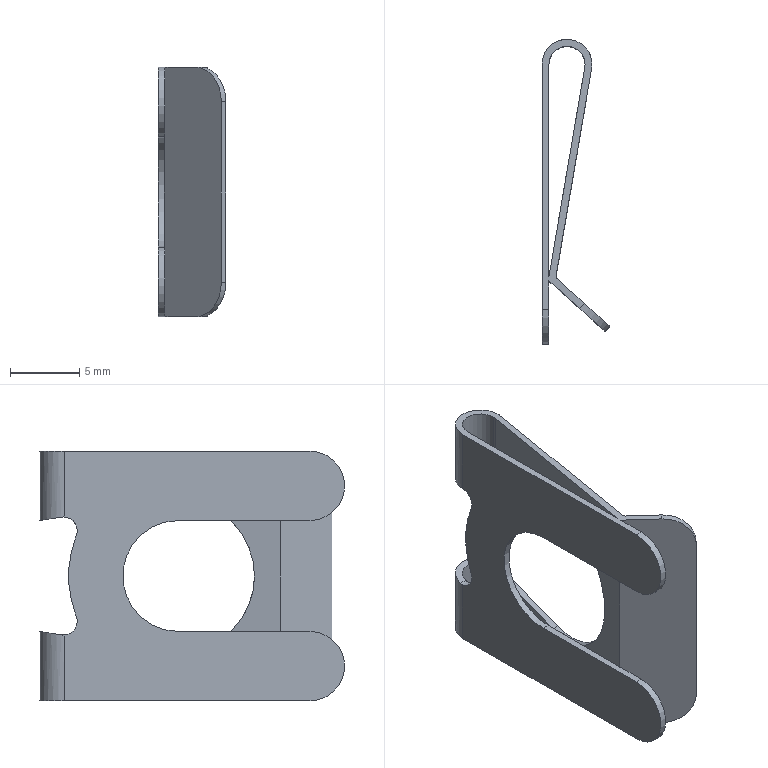Part | SolidWorks | features Fillet 2, BaseBody 1, ICE 1 | 1 solid | 36 faces | box 4.9 x 22 x 18 mm | volume 263.312 mm3 | cylinder 21 | plane 15 | commonest cylinder face diameters 2.6 x4 3.6 x4 5 x4 2 x3 11 x3 0.5 x1
STEP:
#1=CARTESIAN_POINT('',(0.5,8.2,-9.));
#2=VERTEX_POINT('',#1);
#3=CARTESIAN_POINT('',(3.1,8.2,-9.));
#4=VERTEX_POINT('',#3);
#5=CARTESIAN_POINT('',(1.8,8.2,-9.));
#6=DIRECTION('',(0.,0.,-1.));
#7=DIRECTION('',(1.,0.,0.));
#8=AXIS2_PLACEMENT_3D('',#5,#6,#7);
#9=CIRCLE('',#8,1.3);
#10=EDGE_CURVE('',#2,#4,#9,.T.);
#11=ORIENTED_EDGE('',*,*,#10,.T.);
#12=CARTESIAN_POINT('',(3.1,8.2,-4.282));
#13=VERTEX_POINT('',#12);
#14=CARTESIAN_POINT('',(3.1,8.2,9.));
#15=DIRECTION('',(0.,0.,1.));
#16=VECTOR('',#15,1000.);
#17=LINE('',#14,#16);
#18=EDGE_CURVE('',#4,#13,#17,.T.);
#19=ORIENTED_EDGE('',*,*,#18,.T.);
#20=CARTESIAN_POINT('',(0.5,8.2,-4.282));
#21=VERTEX_POINT('',#20);
#22=CARTESIAN_POINT('',(0.5,8.2,-4.282));
#23=CARTESIAN_POINT('',(0.5,10.8,-3.875));
#24=CARTESIAN_POINT('',(3.1,10.8,-3.875));
#25=CARTESIAN_POINT('',(3.1,8.2,-4.282));
#26=(BOUNDED_CURVE()B_SPLINE_CURVE(3,(#22,#23,#24,#25),.UNSPECIFIED.,.F.,.F.)B_SPLINE_CURVE_WITH_KNOTS((4,4),(4.712,7.854),.UNSPECIFIED.)CURVE()GEOMETRIC_REPRESENTATION_ITEM()RATIONAL_B_SPLINE_CURVE((1.,0.3333,0.3333,1.))REPRESENTATION_ITEM(''));
#27=EDGE_CURVE('',#21,#13,#26,.T.);
#28=ORIENTED_EDGE('',*,*,#27,.F.);
#29=CARTESIAN_POINT('',(0.5,8.2,9.));
#30=DIRECTION('',(0.,0.,-1.));
#31=VECTOR('',#30,1000.);
#32=LINE('',#29,#31);
#33=EDGE_CURVE('',#21,#2,#32,.T.);
#34=ORIENTED_EDGE('',*,*,#33,.T.);
#35=EDGE_LOOP('',(#11,#19,#28,#34));
#36=FACE_OUTER_BOUND('',#35,.T.);
#37=CARTESIAN_POINT('',(1.8,8.2,9.));
#38=DIRECTION('',(0.,0.,1.));
#39=DIRECTION('',(1.,0.,0.));
#40=AXIS2_PLACEMENT_3D('',#37,#38,#39);
#41=CYLINDRICAL_SURFACE('',#40,1.3);
#42=ADVANCED_FACE('',(#36),#41,.F.);
#43=CARTESIAN_POINT('',(0.5,8.437,4.245));
#44=VERTEX_POINT('',#43);
#45=CARTESIAN_POINT('',(0.5,8.283,4.257));
#46=VERTEX_POINT('',#45);
#47=CARTESIAN_POINT('',(0.5,8.283,3.257));
#48=DIRECTION('',(1.,0.,0.));
#49=DIRECTION('',(0.,0.,1.));
#50=AXIS2_PLACEMENT_3D('',#47,#48,#49);
#51=CIRCLE('',#50,1.);
#52=EDGE_CURVE('',#44,#46,#51,.T.);
#53=ORIENTED_EDGE('',*,*,#52,.T.);
#54=CARTESIAN_POINT('',(0.001899,8.283,4.257));
#55=VERTEX_POINT('',#54);
#56=CARTESIAN_POINT('',(-4.4,8.283,4.257));
#57=DIRECTION('',(-1.,0.,0.));
#58=VECTOR('',#57,1000.);
#59=LINE('',#56,#58);
#60=EDGE_CURVE('',#46,#55,#59,.T.);
#61=ORIENTED_EDGE('',*,*,#60,.T.);
#62=CARTESIAN_POINT('',(0.01573,8.437,4.245));
#63=VERTEX_POINT('',#62);
#64=CARTESIAN_POINT('',(0.01573,8.437,4.245));
#65=CARTESIAN_POINT('',(0.008933,8.386,4.253));
#66=CARTESIAN_POINT('',(0.004295,8.335,4.257));
#67=CARTESIAN_POINT('',(0.001899,8.283,4.257));
#68=B_SPLINE_CURVE_WITH_KNOTS('',3,(#64,#65,#66,#67),.UNSPECIFIED.,.F.,.F.,(4,4),(-0.0001563,0.),.UNSPECIFIED.);
#69=EDGE_CURVE('',#63,#55,#68,.T.);
#70=ORIENTED_EDGE('',*,*,#69,.F.);
#71=CARTESIAN_POINT('',(5.4,8.437,4.245));
#72=DIRECTION('',(-1.,0.,0.));
#73=VECTOR('',#72,1000.);
#74=LINE('',#71,#73);
#75=EDGE_CURVE('',#44,#63,#74,.T.);
#76=ORIENTED_EDGE('',*,*,#75,.F.);
#77=EDGE_LOOP('',(#53,#61,#70,#76));
#78=FACE_OUTER_BOUND('',#77,.T.);
#79=CARTESIAN_POINT('',(-4.4,8.283,3.257));
#80=DIRECTION('',(-1.,0.,0.));
#81=DIRECTION('',(0.,0.,1.));
#82=AXIS2_PLACEMENT_3D('',#79,#80,#81);
#83=CYLINDRICAL_SURFACE('',#82,1.);
#84=ADVANCED_FACE('',(#78),#83,.F.);
#85=CARTESIAN_POINT('',(3.1,8.2,4.282));
#86=VERTEX_POINT('',#85);
#87=CARTESIAN_POINT('',(0.5,8.2,4.282));
#88=VERTEX_POINT('',#87);
#89=CARTESIAN_POINT('',(3.1,8.2,4.282));
#90=CARTESIAN_POINT('',(3.1,10.8,3.875));
#91=CARTESIAN_POINT('',(0.5,10.8,3.875));
#92=CARTESIAN_POINT('',(0.5,8.2,4.282));
#93=(BOUNDED_CURVE()B_SPLINE_CURVE(3,(#89,#90,#91,#92),.UNSPECIFIED.,.F.,.F.)B_SPLINE_CURVE_WITH_KNOTS((4,4),(1.571,4.712),.UNSPECIFIED.)CURVE()GEOMETRIC_REPRESENTATION_ITEM()RATIONAL_B_SPLINE_CURVE((1.,0.3333,0.3333,1.))REPRESENTATION_ITEM(''));
#94=EDGE_CURVE('',#86,#88,#93,.T.);
#95=ORIENTED_EDGE('',*,*,#94,.F.);
#96=CARTESIAN_POINT('',(3.1,8.2,9.));
#97=VERTEX_POINT('',#96);
#98=CARTESIAN_POINT('',(3.1,8.2,9.));
#99=DIRECTION('',(0.,0.,1.));
#100=VECTOR('',#99,1000.);
#101=LINE('',#98,#100);
#102=EDGE_CURVE('',#86,#97,#101,.T.);
#103=ORIENTED_EDGE('',*,*,#102,.T.);
#104=CARTESIAN_POINT('',(0.5,8.2,9.));
#105=VERTEX_POINT('',#104);
#106=CARTESIAN_POINT('',(1.8,8.2,9.));
#107=DIRECTION('',(0.,0.,-1.));
#108=DIRECTION('',(1.,0.,0.));
#109=AXIS2_PLACEMENT_3D('',#106,#107,#108);
#110=CIRCLE('',#109,1.3);
#111=EDGE_CURVE('',#105,#97,#110,.T.);
#112=ORIENTED_EDGE('',*,*,#111,.F.);
#113=CARTESIAN_POINT('',(0.5,8.2,9.));
#114=DIRECTION('',(0.,0.,-1.));
#115=VECTOR('',#114,1000.);
#116=LINE('',#113,#115);
#117=EDGE_CURVE('',#105,#88,#116,.T.);
#118=ORIENTED_EDGE('',*,*,#117,.T.);
#119=EDGE_LOOP('',(#95,#103,#112,#118));
#120=FACE_OUTER_BOUND('',#119,.T.);
#121=CARTESIAN_POINT('',(1.8,8.2,9.));
#122=DIRECTION('',(0.,0.,1.));
#123=DIRECTION('',(1.,0.,0.));
#124=AXIS2_PLACEMENT_3D('',#121,#122,#123);
#125=CYLINDRICAL_SURFACE('',#124,1.3);
#126=ADVANCED_FACE('',(#120),#125,.F.);
#127=CARTESIAN_POINT('',(3.574,7.896,-9.));
#128=VERTEX_POINT('',#127);
#129=CARTESIAN_POINT('',(3.6,8.2,-9.));
#130=VERTEX_POINT('',#129);
#131=CARTESIAN_POINT('',(1.8,8.2,-9.));
#132=DIRECTION('',(0.,0.,1.));
#133=DIRECTION('',(1.,0.,0.));
#134=AXIS2_PLACEMENT_3D('',#131,#132,#133);
#135=CIRCLE('',#134,1.8);
#136=EDGE_CURVE('',#128,#130,#135,.T.);
#137=ORIENTED_EDGE('',*,*,#136,.T.);
#138=CARTESIAN_POINT('',(3.6,8.2,-4.282));
#139=VERTEX_POINT('',#138);
#140=CARTESIAN_POINT('',(3.6,8.2,9.));
#141=DIRECTION('',(0.,0.,1.));
#142=VECTOR('',#141,1000.);
#143=LINE('',#140,#142);
#144=EDGE_CURVE('',#130,#139,#143,.T.);
#145=ORIENTED_EDGE('',*,*,#144,.T.);
#146=CARTESIAN_POINT('',(3.574,7.896,-4.33));
#147=VERTEX_POINT('',#146);
#148=CARTESIAN_POINT('',(3.6,8.2,-4.282));
#149=CARTESIAN_POINT('',(3.6,8.098,-4.298));
#150=CARTESIAN_POINT('',(3.591,7.997,-4.314));
#151=CARTESIAN_POINT('',(3.574,7.896,-4.33));
#152=(BOUNDED_CURVE()B_SPLINE_CURVE(3,(#148,#149,#150,#151),.UNSPECIFIED.,.F.,.F.)B_SPLINE_CURVE_WITH_KNOTS((4,4),(1.571,1.74),.UNSPECIFIED.)CURVE()GEOMETRIC_REPRESENTATION_ITEM()RATIONAL_B_SPLINE_CURVE((1.,0.9976,0.9976,1.))REPRESENTATION_ITEM(''));
#153=EDGE_CURVE('',#139,#147,#152,.T.);
#154=ORIENTED_EDGE('',*,*,#153,.T.);
#155=CARTESIAN_POINT('',(3.574,7.896,9.));
#156=DIRECTION('',(0.,0.,-1.));
#157=VECTOR('',#156,1000.);
#158=LINE('',#155,#157);
#159=EDGE_CURVE('',#147,#128,#158,.T.);
#160=ORIENTED_EDGE('',*,*,#159,.T.);
#161=EDGE_LOOP('',(#137,#145,#154,#160));
#162=FACE_OUTER_BOUND('',#161,.T.);
#163=CARTESIAN_POINT('',(1.8,8.2,9.));
#164=DIRECTION('',(0.,0.,1.));
#165=DIRECTION('',(1.,0.,0.));
#166=AXIS2_PLACEMENT_3D('',#163,#164,#165);
#167=CYLINDRICAL_SURFACE('',#166,1.8);
#168=ADVANCED_FACE('',(#162),#167,.T.);
#169=CARTESIAN_POINT('',(3.6,8.2,4.282));
#170=VERTEX_POINT('',#169);
#171=CARTESIAN_POINT('',(3.574,7.896,4.33));
#172=VERTEX_POINT('',#171);
#173=CARTESIAN_POINT('',(3.6,8.2,4.282));
#174=CARTESIAN_POINT('',(3.6,8.098,4.298));
#175=CARTESIAN_POINT('',(3.591,7.997,4.314));
#176=CARTESIAN_POINT('',(3.574,7.896,4.33));
#177=(BOUNDED_CURVE()B_SPLINE_CURVE(3,(#173,#174,#175,#176),.UNSPECIFIED.,.F.,.F.)B_SPLINE_CURVE_WITH_KNOTS((4,4),(4.712,4.882),.UNSPECIFIED.)CURVE()GEOMETRIC_REPRESENTATION_ITEM()RATIONAL_B_SPLINE_CURVE((1.,0.9976,0.9976,1.))REPRESENTATION_ITEM(''));
#178=EDGE_CURVE('',#170,#172,#177,.T.);
#179=ORIENTED_EDGE('',*,*,#178,.F.);
#180=CARTESIAN_POINT('',(3.6,8.2,9.));
#181=VERTEX_POINT('',#180);
#182=CARTESIAN_POINT('',(3.6,8.2,9.));
#183=DIRECTION('',(0.,0.,1.));
#184=VECTOR('',#183,1000.);
#185=LINE('',#182,#184);
#186=EDGE_CURVE('',#170,#181,#185,.T.);
#187=ORIENTED_EDGE('',*,*,#186,.T.);
#188=CARTESIAN_POINT('',(3.574,7.896,9.));
#189=VERTEX_POINT('',#188);
#190=CARTESIAN_POINT('',(1.8,8.2,9.));
#191=DIRECTION('',(0.,0.,1.));
#192=DIRECTION('',(1.,0.,0.));
#193=AXIS2_PLACEMENT_3D('',#190,#191,#192);
#194=CIRCLE('',#193,1.8);
#195=EDGE_CURVE('',#189,#181,#194,.T.);
#196=ORIENTED_EDGE('',*,*,#195,.F.);
#197=CARTESIAN_POINT('',(3.574,7.896,9.));
#198=DIRECTION('',(0.,0.,-1.));
#199=VECTOR('',#198,1000.);
#200=LINE('',#197,#199);
#201=EDGE_CURVE('',#189,#172,#200,.T.);
#202=ORIENTED_EDGE('',*,*,#201,.T.);
#203=EDGE_LOOP('',(#179,#187,#196,#202));
#204=FACE_OUTER_BOUND('',#203,.T.);
#205=CARTESIAN_POINT('',(1.8,8.2,9.));
#206=DIRECTION('',(0.,0.,1.));
#207=DIRECTION('',(1.,0.,0.));
#208=AXIS2_PLACEMENT_3D('',#205,#206,#207);
#209=CYLINDRICAL_SURFACE('',#208,1.8);
#210=ADVANCED_FACE('',(#204),#209,.T.);
#211=CARTESIAN_POINT('',(1.715,0.,-5.5));
#212=VERTEX_POINT('',#211);
#213=CARTESIAN_POINT('',(1.715,0.,5.5));
#214=VERTEX_POINT('',#213);
#215=CARTESIAN_POINT('',(1.715,0.,-5.5));
#216=CARTESIAN_POINT('',(-0.1676,-11.,-5.5));
#217=CARTESIAN_POINT('',(-0.1676,-11.,5.5));
#218=CARTESIAN_POINT('',(1.715,0.,5.5));
#219=(BOUNDED_CURVE()B_SPLINE_CURVE(3,(#215,#216,#217,#218),.UNSPECIFIED.,.F.,.F.)B_SPLINE_CURVE_WITH_KNOTS((4,4),(1.571,4.712),.UNSPECIFIED.)CURVE()GEOMETRIC_REPRESENTATION_ITEM()RATIONAL_B_SPLINE_CURVE((1.,0.3333,0.3333,1.))REPRESENTATION_ITEM(''));
#220=EDGE_CURVE('',#212,#214,#219,.T.);
#221=ORIENTED_EDGE('',*,*,#220,.T.);
#222=CARTESIAN_POINT('',(2.223,0.,5.5));
#223=VERTEX_POINT('',#222);
#224=CARTESIAN_POINT('',(5.4,0.,5.5));
#225=DIRECTION('',(1.,0.,0.));
#226=VECTOR('',#225,1000.);
#227=LINE('',#224,#226);
#228=EDGE_CURVE('',#214,#223,#227,.T.);
#229=ORIENTED_EDGE('',*,*,#228,.T.);
#230=CARTESIAN_POINT('',(2.223,0.,-5.5));
#231=VERTEX_POINT('',#230);
#232=CARTESIAN_POINT('',(2.223,0.,5.5));
#233=CARTESIAN_POINT('',(0.3397,-11.,5.5));
#234=CARTESIAN_POINT('',(0.3397,-11.,-5.5));
#235=CARTESIAN_POINT('',(2.223,0.,-5.5));
#236=(BOUNDED_CURVE()B_SPLINE_CURVE(3,(#232,#233,#234,#235),.UNSPECIFIED.,.F.,.F.)B_SPLINE_CURVE_WITH_KNOTS((4,4),(1.571,4.712),.UNSPECIFIED.)CURVE()GEOMETRIC_REPRESENTATION_ITEM()RATIONAL_B_SPLINE_CURVE((1.,0.3333,0.3333,1.))REPRESENTATION_ITEM(''));
#237=EDGE_CURVE('',#223,#231,#236,.T.);
#238=ORIENTED_EDGE('',*,*,#237,.T.);
#239=CARTESIAN_POINT('',(5.4,0.,-5.5));
#240=DIRECTION('',(1.,0.,0.));
#241=VECTOR('',#240,1000.);
#242=LINE('',#239,#241);
#243=EDGE_CURVE('',#212,#231,#242,.T.);
#244=ORIENTED_EDGE('',*,*,#243,.F.);
#245=EDGE_LOOP('',(#221,#229,#238,#244));
#246=FACE_OUTER_BOUND('',#245,.T.);
#247=CARTESIAN_POINT('',(5.4,0.,0.));
#248=DIRECTION('',(1.,0.,0.));
#249=DIRECTION('',(0.,0.,-1.));
#250=AXIS2_PLACEMENT_3D('',#247,#248,#249);
#251=CYLINDRICAL_SURFACE('',#250,5.5);
#252=ADVANCED_FACE('',(#246),#251,.F.);
#253=CARTESIAN_POINT('',(1.861,0.8515,-5.434));
#254=VERTEX_POINT('',#253);
#255=CARTESIAN_POINT('',(1.861,0.8515,-5.434));
#256=CARTESIAN_POINT('',(1.813,0.5697,-5.478));
#257=CARTESIAN_POINT('',(1.764,0.2853,-5.5));
#258=CARTESIAN_POINT('',(1.715,0.,-5.5));
#259=(BOUNDED_CURVE()B_SPLINE_CURVE(3,(#255,#256,#257,#258),.UNSPECIFIED.,.F.,.F.)B_SPLINE_CURVE_WITH_KNOTS((4,4),(1.415,1.571),.UNSPECIFIED.)CURVE()GEOMETRIC_REPRESENTATION_ITEM()RATIONAL_B_SPLINE_CURVE((1.,0.998,0.998,1.))REPRESENTATION_ITEM(''));
#260=EDGE_CURVE('',#254,#212,#259,.T.);
#261=ORIENTED_EDGE('',*,*,#260,.T.);
#262=ORIENTED_EDGE('',*,*,#243,.T.);
#263=CARTESIAN_POINT('',(2.368,0.8515,-5.434));
#264=VERTEX_POINT('',#263);
#265=CARTESIAN_POINT('',(2.223,0.,-5.5));
#266=CARTESIAN_POINT('',(2.271,0.2853,-5.5));
#267=CARTESIAN_POINT('',(2.32,0.5697,-5.478));
#268=CARTESIAN_POINT('',(2.368,0.8515,-5.434));
#269=(BOUNDED_CURVE()B_SPLINE_CURVE(3,(#265,#266,#267,#268),.UNSPECIFIED.,.F.,.F.)B_SPLINE_CURVE_WITH_KNOTS((4,4),(4.712,4.868),.UNSPECIFIED.)CURVE()GEOMETRIC_REPRESENTATION_ITEM()RATIONAL_B_SPLINE_CURVE((1.,0.998,0.998,1.))REPRESENTATION_ITEM(''));
#270=EDGE_CURVE('',#231,#264,#269,.T.);
#271=ORIENTED_EDGE('',*,*,#270,.T.);
#272=CARTESIAN_POINT('',(5.4,0.8515,-5.434));
#273=DIRECTION('',(1.,0.,0.));
#274=VECTOR('',#273,1000.);
#275=LINE('',#272,#274);
#276=EDGE_CURVE('',#254,#264,#275,.T.);
#277=ORIENTED_EDGE('',*,*,#276,.F.);
#278=EDGE_LOOP('',(#261,#262,#271,#277));
#279=FACE_OUTER_BOUND('',#278,.T.);
#280=CARTESIAN_POINT('',(5.4,0.,0.));
#281=DIRECTION('',(1.,0.,0.));
#282=DIRECTION('',(0.,0.,-1.));
#283=AXIS2_PLACEMENT_3D('',#280,#281,#282);
#284=CYLINDRICAL_SURFACE('',#283,5.5);
#285=ADVANCED_FACE('',(#279),#284,.F.);
#286=CARTESIAN_POINT('',(4.565,-11.072,6.5));
#287=VERTEX_POINT('',#286);
#288=CARTESIAN_POINT('',(4.565,-11.072,-6.5));
#289=VERTEX_POINT('',#288);
#290=CARTESIAN_POINT('',(4.565,-11.072,-9.));
#291=DIRECTION('',(0.,0.,-1.));
#292=VECTOR('',#291,1000.);
#293=LINE('',#290,#292);
#294=EDGE_CURVE('',#287,#289,#293,.T.);
#295=ORIENTED_EDGE('',*,*,#294,.F.);
#296=CARTESIAN_POINT('',(2.707,-9.399,9.));
#297=VERTEX_POINT('',#296);
#298=CARTESIAN_POINT('',(2.707,-9.399,6.5));
#299=DIRECTION('',(-0.6689,-0.7434,0.));
#300=DIRECTION('',(-0.7434,0.6689,0.));
#301=AXIS2_PLACEMENT_3D('',#298,#299,#300);
#302=CIRCLE('',#301,2.5);
#303=EDGE_CURVE('',#287,#297,#302,.T.);
#304=ORIENTED_EDGE('',*,*,#303,.T.);
#305=CARTESIAN_POINT('',(0.5,-7.414,9.));
#306=VERTEX_POINT('',#305);
#307=CARTESIAN_POINT('',(0.7608,-7.648,9.));
#308=DIRECTION('',(0.7434,-0.6689,0.));
#309=VECTOR('',#308,1000.);
#310=LINE('',#307,#309);
#311=EDGE_CURVE('',#306,#297,#310,.T.);
#312=ORIENTED_EDGE('',*,*,#311,.F.);
#313=CARTESIAN_POINT('',(0.5,-7.414,4.));
#314=VERTEX_POINT('',#313);
#315=CARTESIAN_POINT('',(0.5,-7.414,9.));
#316=DIRECTION('',(0.,0.,1.));
#317=VECTOR('',#316,1000.);
#318=LINE('',#315,#317);
#319=EDGE_CURVE('',#314,#306,#318,.T.);
#320=ORIENTED_EDGE('',*,*,#319,.F.);
#321=CARTESIAN_POINT('',(0.4535,-7.372,4.));
#322=VERTEX_POINT('',#321);
#323=CARTESIAN_POINT('',(0.7608,-7.648,4.));
#324=DIRECTION('',(-0.7434,0.6689,0.));
#325=VECTOR('',#324,1000.);
#326=LINE('',#323,#325);
#327=EDGE_CURVE('',#314,#322,#326,.T.);
#328=ORIENTED_EDGE('',*,*,#327,.T.);
#329=CARTESIAN_POINT('',(0.4535,-7.372,-4.));
#330=VERTEX_POINT('',#329);
#331=CARTESIAN_POINT('',(0.4535,-7.372,9.));
#332=DIRECTION('',(0.,0.,-1.));
#333=VECTOR('',#332,1000.);
#334=LINE('',#331,#333);
#335=EDGE_CURVE('',#322,#330,#334,.T.);
#336=ORIENTED_EDGE('',*,*,#335,.T.);
#337=CARTESIAN_POINT('',(0.5,-7.414,-4.));
#338=VERTEX_POINT('',#337);
#339=CARTESIAN_POINT('',(0.7608,-7.648,-4.));
#340=DIRECTION('',(0.7434,-0.6689,0.));
#341=VECTOR('',#340,1000.);
#342=LINE('',#339,#341);
#343=EDGE_CURVE('',#330,#338,#342,.T.);
#344=ORIENTED_EDGE('',*,*,#343,.T.);
#345=CARTESIAN_POINT('',(0.5,-7.414,-9.));
#346=VERTEX_POINT('',#345);
#347=CARTESIAN_POINT('',(0.5,-7.414,9.));
#348=DIRECTION('',(0.,0.,1.));
#349=VECTOR('',#348,1000.);
#350=LINE('',#347,#349);
#351=EDGE_CURVE('',#346,#338,#350,.T.);
#352=ORIENTED_EDGE('',*,*,#351,.F.);
#353=CARTESIAN_POINT('',(2.707,-9.399,-9.));
#354=VERTEX_POINT('',#353);
#355=CARTESIAN_POINT('',(0.7608,-7.648,-9.));
#356=DIRECTION('',(0.7434,-0.6689,0.));
#357=VECTOR('',#356,1000.);
#358=LINE('',#355,#357);
#359=EDGE_CURVE('',#346,#354,#358,.T.);
#360=ORIENTED_EDGE('',*,*,#359,.T.);
#361=CARTESIAN_POINT('',(2.707,-9.399,-6.5));
#362=DIRECTION('',(-0.6689,-0.7434,0.));
#363=DIRECTION('',(-0.7434,0.6689,0.));
#364=AXIS2_PLACEMENT_3D('',#361,#362,#363);
#365=CIRCLE('',#364,2.5);
#366=EDGE_CURVE('',#354,#289,#365,.T.);
#367=ORIENTED_EDGE('',*,*,#366,.T.);
#368=EDGE_LOOP('',(#295,#304,#312,#320,#328,#336,#344,#352,#360,#367));
#369=FACE_OUTER_BOUND('',#368,.T.);
#370=CARTESIAN_POINT('',(0.7608,-7.648,9.));
#371=DIRECTION('',(0.6689,0.7434,0.));
#372=DIRECTION('',(0.,0.,-1.));
#373=AXIS2_PLACEMENT_3D('',#370,#371,#372);
#374=PLANE('',#373);
#375=ADVANCED_FACE('',(#369),#374,.F.);
#376=CARTESIAN_POINT('',(3.081,7.981,9.));
#377=VERTEX_POINT('',#376);
#378=CARTESIAN_POINT('',(0.5,-7.1,9.));
#379=VERTEX_POINT('',#378);
#380=CARTESIAN_POINT('',(3.081,7.981,9.));
#381=DIRECTION('',(-0.1687,-0.9857,0.));
#382=VECTOR('',#381,1000.);
#383=LINE('',#380,#382);
#384=EDGE_CURVE('',#377,#379,#383,.T.);
#385=ORIENTED_EDGE('',*,*,#384,.T.);
#386=CARTESIAN_POINT('',(0.5,-12.,9.));
#387=DIRECTION('',(0.,1.,0.));
#388=VECTOR('',#387,1000.);
#389=LINE('',#386,#388);
#390=EDGE_CURVE('',#379,#105,#389,.T.);
#391=ORIENTED_EDGE('',*,*,#390,.T.);
#392=ORIENTED_EDGE('',*,*,#111,.T.);
#393=CARTESIAN_POINT('',(1.8,8.2,9.));
#394=DIRECTION('',(0.,0.,-1.));
#395=DIRECTION('',(1.,0.,0.));
#396=AXIS2_PLACEMENT_3D('',#393,#394,#395);
#397=CIRCLE('',#396,1.3);
#398=EDGE_CURVE('',#97,#377,#397,.T.);
#399=ORIENTED_EDGE('',*,*,#398,.T.);
#400=EDGE_LOOP('',(#385,#391,#392,#399));
#401=FACE_BOUND('',#400,.T.);
#402=ORIENTED_EDGE('',*,*,#311,.T.);
#403=CARTESIAN_POINT('',(3.041,-9.028,9.));
#404=VERTEX_POINT('',#403);
#405=CARTESIAN_POINT('',(3.041,-9.028,9.));
#406=DIRECTION('',(0.6689,0.7434,0.));
#407=VECTOR('',#406,1000.);
#408=LINE('',#405,#407);
#409=EDGE_CURVE('',#297,#404,#408,.T.);
#410=ORIENTED_EDGE('',*,*,#409,.T.);
#411=CARTESIAN_POINT('',(1.095,-7.277,9.));
#412=VERTEX_POINT('',#411);
#413=CARTESIAN_POINT('',(4.9,-10.7,9.));
#414=DIRECTION('',(-0.7434,0.6689,0.));
#415=VECTOR('',#414,1000.);
#416=LINE('',#413,#415);
#417=EDGE_CURVE('',#404,#412,#416,.T.);
#418=ORIENTED_EDGE('',*,*,#417,.T.);
#419=CARTESIAN_POINT('',(1.016,-7.049,9.));
#420=VERTEX_POINT('',#419);
#421=CARTESIAN_POINT('',(1.263,-7.091,9.));
#422=DIRECTION('',(0.,0.,-1.));
#423=DIRECTION('',(1.,0.,0.));
#424=AXIS2_PLACEMENT_3D('',#421,#422,#423);
#425=CIRCLE('',#424,0.25);
#426=EDGE_CURVE('',#412,#420,#425,.T.);
#427=ORIENTED_EDGE('',*,*,#426,.T.);
#428=CARTESIAN_POINT('',(1.016,-7.049,9.));
#429=DIRECTION('',(0.1687,0.9857,0.));
#430=VECTOR('',#429,1000.);
#431=LINE('',#428,#430);
#432=EDGE_CURVE('',#420,#189,#431,.T.);
#433=ORIENTED_EDGE('',*,*,#432,.T.);
#434=ORIENTED_EDGE('',*,*,#195,.T.);
#435=CARTESIAN_POINT('',(0.,8.2,9.));
#436=VERTEX_POINT('',#435);
#437=CARTESIAN_POINT('',(1.8,8.2,9.));
#438=DIRECTION('',(0.,0.,1.));
#439=DIRECTION('',(1.,0.,0.));
#440=AXIS2_PLACEMENT_3D('',#437,#438,#439);
#441=CIRCLE('',#440,1.8);
#442=EDGE_CURVE('',#181,#436,#441,.T.);
#443=ORIENTED_EDGE('',*,*,#442,.T.);
#444=CARTESIAN_POINT('',(0.,-9.5,9.));
#445=VERTEX_POINT('',#444);
#446=CARTESIAN_POINT('',(0.,8.2,9.));
#447=DIRECTION('',(0.,-1.,0.));
#448=VECTOR('',#447,1000.);
#449=LINE('',#446,#448);
#450=EDGE_CURVE('',#436,#445,#449,.T.);
#451=ORIENTED_EDGE('',*,*,#450,.T.);
#452=CARTESIAN_POINT('',(0.5,-9.5,9.));
#453=VERTEX_POINT('',#452);
#454=CARTESIAN_POINT('',(1.8,-9.5,9.));
#455=DIRECTION('',(1.,0.,0.));
#456=VECTOR('',#455,1000.);
#457=LINE('',#454,#456);
#458=EDGE_CURVE('',#445,#453,#457,.T.);
#459=ORIENTED_EDGE('',*,*,#458,.T.);
#460=CARTESIAN_POINT('',(0.5,-12.,9.));
#461=DIRECTION('',(0.,1.,0.));
#462=VECTOR('',#461,1000.);
#463=LINE('',#460,#462);
#464=EDGE_CURVE('',#453,#306,#463,.T.);
#465=ORIENTED_EDGE('',*,*,#464,.T.);
#466=EDGE_LOOP('',(#402,#410,#418,#427,#433,#434,#443,#451,#459,#465));
#467=FACE_OUTER_BOUND('',#466,.T.);
#468=CARTESIAN_POINT('',(1.8,8.2,9.));
#469=DIRECTION('',(0.,0.,1.));
#470=DIRECTION('',(1.,0.,0.));
#471=AXIS2_PLACEMENT_3D('',#468,#469,#470);
#472=PLANE('',#471);
#473=ADVANCED_FACE('',(#401,#467),#472,.T.);
#474=CARTESIAN_POINT('',(0.5,-7.1,-9.));
#475=VERTEX_POINT('',#474);
#476=CARTESIAN_POINT('',(0.5,-12.,-9.));
#477=DIRECTION('',(0.,-1.,0.));
#478=VECTOR('',#477,1000.);
#479=LINE('',#476,#478);
#480=EDGE_CURVE('',#2,#475,#479,.T.);
#481=ORIENTED_EDGE('',*,*,#480,.T.);
#482=CARTESIAN_POINT('',(3.081,7.981,-9.));
#483=VERTEX_POINT('',#482);
#484=CARTESIAN_POINT('',(3.081,7.981,-9.));
#485=DIRECTION('',(-0.1687,-0.9857,0.));
#486=VECTOR('',#485,1000.);
#487=LINE('',#484,#486);
#488=EDGE_CURVE('',#483,#475,#487,.T.);
#489=ORIENTED_EDGE('',*,*,#488,.F.);
#490=CARTESIAN_POINT('',(1.8,8.2,-9.));
#491=DIRECTION('',(0.,0.,-1.));
#492=DIRECTION('',(1.,0.,0.));
#493=AXIS2_PLACEMENT_3D('',#490,#491,#492);
#494=CIRCLE('',#493,1.3);
#495=EDGE_CURVE('',#4,#483,#494,.T.);
#496=ORIENTED_EDGE('',*,*,#495,.F.);
#497=ORIENTED_EDGE('',*,*,#10,.F.);
#498=EDGE_LOOP('',(#481,#489,#496,#497));
#499=FACE_BOUND('',#498,.T.);
#500=CARTESIAN_POINT('',(3.041,-9.028,-9.));
#501=VERTEX_POINT('',#500);
#502=CARTESIAN_POINT('',(1.095,-7.277,-9.));
#503=VERTEX_POINT('',#502);
#504=CARTESIAN_POINT('',(4.9,-10.7,-9.));
#505=DIRECTION('',(-0.7434,0.6689,0.));
#506=VECTOR('',#505,1000.);
#507=LINE('',#504,#506);
#508=EDGE_CURVE('',#501,#503,#507,.T.);
#509=ORIENTED_EDGE('',*,*,#508,.F.);
#510=CARTESIAN_POINT('',(11.052,-0.1249,-9.));
#511=DIRECTION('',(-0.6689,-0.7434,0.));
#512=VECTOR('',#511,1000.);
#513=LINE('',#510,#512);
#514=EDGE_CURVE('',#501,#354,#513,.T.);
#515=ORIENTED_EDGE('',*,*,#514,.T.);
#516=ORIENTED_EDGE('',*,*,#359,.F.);
#517=CARTESIAN_POINT('',(0.5,-9.5,-9.));
#518=VERTEX_POINT('',#517);
#519=CARTESIAN_POINT('',(0.5,-12.,-9.));
#520=DIRECTION('',(0.,-1.,0.));
#521=VECTOR('',#520,1000.);
#522=LINE('',#519,#521);
#523=EDGE_CURVE('',#346,#518,#522,.T.);
#524=ORIENTED_EDGE('',*,*,#523,.T.);
#525=CARTESIAN_POINT('',(0.,-9.5,-9.));
#526=VERTEX_POINT('',#525);
#527=CARTESIAN_POINT('',(0.5,-9.5,-9.));
#528=DIRECTION('',(1.,0.,0.));
#529=VECTOR('',#528,1000.);
#530=LINE('',#527,#529);
#531=EDGE_CURVE('',#526,#518,#530,.T.);
#532=ORIENTED_EDGE('',*,*,#531,.F.);
#533=CARTESIAN_POINT('',(0.,8.2,-9.));
#534=VERTEX_POINT('',#533);
#535=CARTESIAN_POINT('',(0.,8.2,-9.));
#536=DIRECTION('',(0.,-1.,0.));
#537=VECTOR('',#536,1000.);
#538=LINE('',#535,#537);
#539=EDGE_CURVE('',#534,#526,#538,.T.);
#540=ORIENTED_EDGE('',*,*,#539,.F.);
#541=CARTESIAN_POINT('',(1.8,8.2,-9.));
#542=DIRECTION('',(0.,0.,1.));
#543=DIRECTION('',(1.,0.,0.));
#544=AXIS2_PLACEMENT_3D('',#541,#542,#543);
#545=CIRCLE('',#544,1.8);
#546=EDGE_CURVE('',#130,#534,#545,.T.);
#547=ORIENTED_EDGE('',*,*,#546,.F.);
#548=ORIENTED_EDGE('',*,*,#136,.F.);
#549=CARTESIAN_POINT('',(1.016,-7.049,-9.));
#550=VERTEX_POINT('',#549);
#551=CARTESIAN_POINT('',(1.016,-7.049,-9.));
#552=DIRECTION('',(0.1687,0.9857,0.));
#553=VECTOR('',#552,1000.);
#554=LINE('',#551,#553);
#555=EDGE_CURVE('',#550,#128,#554,.T.);
#556=ORIENTED_EDGE('',*,*,#555,.F.);
#557=CARTESIAN_POINT('',(1.263,-7.091,-9.));
#558=DIRECTION('',(0.,0.,1.));
#559=DIRECTION('',(1.,0.,0.));
#560=AXIS2_PLACEMENT_3D('',#557,#558,#559);
#561=CIRCLE('',#560,0.25);
#562=EDGE_CURVE('',#550,#503,#561,.T.);
#563=ORIENTED_EDGE('',*,*,#562,.T.);
#564=EDGE_LOOP('',(#509,#515,#516,#524,#532,#540,#547,#548,#556,#563));
#565=FACE_OUTER_BOUND('',#564,.T.);
#566=CARTESIAN_POINT('',(1.8,8.2,-9.));
#567=DIRECTION('',(0.,0.,1.));
#568=DIRECTION('',(1.,0.,0.));
#569=AXIS2_PLACEMENT_3D('',#566,#567,#568);
#570=PLANE('',#569);
#571=ADVANCED_FACE('',(#499,#565),#570,.F.);
#572=CARTESIAN_POINT('',(0.5,-7.1,-4.));
#573=VERTEX_POINT('',#572);
#574=CARTESIAN_POINT('',(-0.3149,-11.861,-4.));
#575=DIRECTION('',(0.1687,0.9857,0.));
#576=VECTOR('',#575,1000.);
#577=LINE('',#574,#576);
#578=EDGE_CURVE('',#330,#573,#577,.T.);
#579=ORIENTED_EDGE('',*,*,#578,.F.);
#580=ORIENTED_EDGE('',*,*,#335,.F.);
#581=CARTESIAN_POINT('',(0.5,-7.1,4.));
#582=VERTEX_POINT('',#581);
#583=CARTESIAN_POINT('',(1.681,-0.2021,4.));
#584=DIRECTION('',(-0.1687,-0.9857,0.));
#585=VECTOR('',#584,1000.);
#586=LINE('',#583,#585);
#587=EDGE_CURVE('',#582,#322,#586,.T.);
#588=ORIENTED_EDGE('',*,*,#587,.F.);
#589=CARTESIAN_POINT('',(0.5,-7.1,9.));
#590=DIRECTION('',(0.,0.,1.));
#591=VECTOR('',#590,1000.);
#592=LINE('',#589,#591);
#593=EDGE_CURVE('',#582,#379,#592,.T.);
#594=ORIENTED_EDGE('',*,*,#593,.T.);
#595=ORIENTED_EDGE('',*,*,#384,.F.);
#596=CARTESIAN_POINT('',(3.081,7.981,4.316));
#597=VERTEX_POINT('',#596);
#598=CARTESIAN_POINT('',(3.081,7.981,9.));
#599=DIRECTION('',(0.,0.,1.));
#600=VECTOR('',#599,1000.);
#601=LINE('',#598,#600);
#602=EDGE_CURVE('',#597,#377,#601,.T.);
#603=ORIENTED_EDGE('',*,*,#602,.F.);
#604=CARTESIAN_POINT('',(1.861,0.8515,5.434));
#605=VERTEX_POINT('',#604);
#606=CARTESIAN_POINT('',(1.861,0.8515,5.434));
#607=DIRECTION('',(0.1667,0.9741,-0.1527));
#608=VECTOR('',#607,1000.);
#609=LINE('',#606,#608);
#610=EDGE_CURVE('',#605,#597,#609,.T.);
#611=ORIENTED_EDGE('',*,*,#610,.F.);
#612=CARTESIAN_POINT('',(1.715,0.,5.5));
#613=CARTESIAN_POINT('',(1.764,0.2853,5.5));
#614=CARTESIAN_POINT('',(1.813,0.5697,5.478));
#615=CARTESIAN_POINT('',(1.861,0.8515,5.434));
#616=(BOUNDED_CURVE()B_SPLINE_CURVE(3,(#612,#613,#614,#615),.UNSPECIFIED.,.F.,.F.)B_SPLINE_CURVE_WITH_KNOTS((4,4),(4.712,4.868),.UNSPECIFIED.)CURVE()GEOMETRIC_REPRESENTATION_ITEM()RATIONAL_B_SPLINE_CURVE((1.,0.998,0.998,1.))REPRESENTATION_ITEM(''));
#617=EDGE_CURVE('',#214,#605,#616,.T.);
#618=ORIENTED_EDGE('',*,*,#617,.F.);
#619=ORIENTED_EDGE('',*,*,#220,.F.);
#620=ORIENTED_EDGE('',*,*,#260,.F.);
#621=CARTESIAN_POINT('',(3.081,7.981,-4.316));
#622=VERTEX_POINT('',#621);
#623=CARTESIAN_POINT('',(3.081,7.981,-4.316));
#624=DIRECTION('',(-0.1667,-0.9741,-0.1527));
#625=VECTOR('',#624,1000.);
#626=LINE('',#623,#625);
#627=EDGE_CURVE('',#622,#254,#626,.T.);
#628=ORIENTED_EDGE('',*,*,#627,.F.);
#629=CARTESIAN_POINT('',(3.081,7.981,9.));
#630=DIRECTION('',(0.,0.,1.));
#631=VECTOR('',#630,1000.);
#632=LINE('',#629,#631);
#633=EDGE_CURVE('',#483,#622,#632,.T.);
#634=ORIENTED_EDGE('',*,*,#633,.F.);
#635=ORIENTED_EDGE('',*,*,#488,.T.);
#636=CARTESIAN_POINT('',(0.5,-7.1,9.));
#637=DIRECTION('',(0.,0.,1.));
#638=VECTOR('',#637,1000.);
#639=LINE('',#636,#638);
#640=EDGE_CURVE('',#475,#573,#639,.T.);
#641=ORIENTED_EDGE('',*,*,#640,.T.);
#642=EDGE_LOOP('',(#579,#580,#588,#594,#595,#603,#611,#618,#619,#620,#628,#634,#635,#641));
#643=FACE_OUTER_BOUND('',#642,.T.);
#644=CARTESIAN_POINT('',(3.081,7.981,9.));
#645=DIRECTION('',(0.9857,-0.1687,0.));
#646=DIRECTION('',(0.,0.,-1.));
#647=AXIS2_PLACEMENT_3D('',#644,#645,#646);
#648=PLANE('',#647);
#649=ADVANCED_FACE('',(#643),#648,.F.);
#650=ORIENTED_EDGE('',*,*,#640,.F.);
#651=ORIENTED_EDGE('',*,*,#480,.F.);
#652=ORIENTED_EDGE('',*,*,#33,.F.);
#653=CARTESIAN_POINT('',(0.5,8.437,-4.245));
#654=VERTEX_POINT('',#653);
#655=CARTESIAN_POINT('',(0.5,0.8515,-5.434));
#656=DIRECTION('',(0.,-0.9879,-0.1548));
#657=VECTOR('',#656,1000.);
#658=LINE('',#655,#657);
#659=EDGE_CURVE('',#654,#21,#658,.T.);
#660=ORIENTED_EDGE('',*,*,#659,.F.);
#661=CARTESIAN_POINT('',(0.5,7.352,-2.891));
#662=VERTEX_POINT('',#661);
#663=CARTESIAN_POINT('',(0.5,8.283,-3.257));
#664=DIRECTION('',(1.,0.,0.));
#665=DIRECTION('',(0.,0.,1.));
#666=AXIS2_PLACEMENT_3D('',#663,#664,#665);
#667=CIRCLE('',#666,1.);
#668=EDGE_CURVE('',#662,#654,#667,.T.);
#669=ORIENTED_EDGE('',*,*,#668,.F.);
#670=CARTESIAN_POINT('',(0.5,7.352,2.891));
#671=VERTEX_POINT('',#670);
#672=CARTESIAN_POINT('',(0.5,0.,0.));
#673=DIRECTION('',(-1.,0.,0.));
#674=DIRECTION('',(0.,0.,1.));
#675=AXIS2_PLACEMENT_3D('',#672,#673,#674);
#676=CIRCLE('',#675,7.9);
#677=EDGE_CURVE('',#671,#662,#676,.T.);
#678=ORIENTED_EDGE('',*,*,#677,.F.);
#679=CARTESIAN_POINT('',(0.5,8.283,3.257));
#680=DIRECTION('',(1.,0.,0.));
#681=DIRECTION('',(0.,0.,1.));
#682=AXIS2_PLACEMENT_3D('',#679,#680,#681);
#683=CIRCLE('',#682,1.);
#684=EDGE_CURVE('',#46,#671,#683,.T.);
#685=ORIENTED_EDGE('',*,*,#684,.F.);
#686=ORIENTED_EDGE('',*,*,#52,.F.);
#687=CARTESIAN_POINT('',(0.5,10.,4.));
#688=DIRECTION('',(0.,0.9879,-0.1548));
#689=VECTOR('',#688,1000.);
#690=LINE('',#687,#689);
#691=EDGE_CURVE('',#88,#44,#690,.T.);
#692=ORIENTED_EDGE('',*,*,#691,.F.);
#693=ORIENTED_EDGE('',*,*,#117,.F.);
#694=ORIENTED_EDGE('',*,*,#390,.F.);
#695=ORIENTED_EDGE('',*,*,#593,.F.);
#696=CARTESIAN_POINT('',(0.5,0.,4.));
#697=VERTEX_POINT('',#696);
#698=CARTESIAN_POINT('',(0.5,-12.,4.));
#699=DIRECTION('',(0.,-1.,0.));
#700=VECTOR('',#699,1000.);
#701=LINE('',#698,#700);
#702=EDGE_CURVE('',#697,#582,#701,.T.);
#703=ORIENTED_EDGE('',*,*,#702,.F.);
#704=CARTESIAN_POINT('',(0.5,0.,-4.));
#705=VERTEX_POINT('',#704);
#706=CARTESIAN_POINT('',(0.5,0.,0.));
#707=DIRECTION('',(1.,0.,0.));
#708=DIRECTION('',(0.,0.,-1.));
#709=AXIS2_PLACEMENT_3D('',#706,#707,#708);
#710=CIRCLE('',#709,4.);
#711=EDGE_CURVE('',#705,#697,#710,.T.);
#712=ORIENTED_EDGE('',*,*,#711,.F.);
#713=CARTESIAN_POINT('',(0.5,-12.,-4.));
#714=DIRECTION('',(0.,1.,0.));
#715=VECTOR('',#714,1000.);
#716=LINE('',#713,#715);
#717=EDGE_CURVE('',#573,#705,#716,.T.);
#718=ORIENTED_EDGE('',*,*,#717,.F.);
#719=EDGE_LOOP('',(#650,#651,#652,#660,#669,#678,#685,#686,#692,#693,#694,#695,#703,#712,#718));
#720=FACE_OUTER_BOUND('',#719,.T.);
#721=CARTESIAN_POINT('',(0.5,-12.,9.));
#722=DIRECTION('',(-1.,0.,0.));
#723=DIRECTION('',(0.,0.,1.));
#724=AXIS2_PLACEMENT_3D('',#721,#722,#723);
#725=PLANE('',#724);
#726=ADVANCED_FACE('',(#720),#725,.F.);
#727=ORIENTED_EDGE('',*,*,#523,.F.);
#728=ORIENTED_EDGE('',*,*,#351,.T.);
#729=CARTESIAN_POINT('',(0.5,-9.5,-4.));
#730=VERTEX_POINT('',#729);
#731=CARTESIAN_POINT('',(0.5,-12.,-4.));
#732=DIRECTION('',(0.,1.,0.));
#733=VECTOR('',#732,1000.);
#734=LINE('',#731,#733);
#735=EDGE_CURVE('',#730,#338,#734,.T.);
#736=ORIENTED_EDGE('',*,*,#735,.F.);
#737=CARTESIAN_POINT('',(0.5,-9.5,-6.5));
#738=DIRECTION('',(-1.,0.,0.));
#739=DIRECTION('',(0.,0.,-1.));
#740=AXIS2_PLACEMENT_3D('',#737,#738,#739);
#741=CIRCLE('',#740,2.5);
#742=EDGE_CURVE('',#518,#730,#741,.T.);
#743=ORIENTED_EDGE('',*,*,#742,.F.);
#744=EDGE_LOOP('',(#727,#728,#736,#743));
#745=FACE_OUTER_BOUND('',#744,.T.);
#746=CARTESIAN_POINT('',(0.5,-12.,9.));
#747=DIRECTION('',(-1.,0.,0.));
#748=DIRECTION('',(0.,0.,1.));
#749=AXIS2_PLACEMENT_3D('',#746,#747,#748);
#750=PLANE('',#749);
#751=ADVANCED_FACE('',(#745),#750,.F.);
#752=CARTESIAN_POINT('',(2.368,0.8515,5.434));
#753=VERTEX_POINT('',#752);
#754=CARTESIAN_POINT('',(3.574,7.896,4.33));
#755=DIRECTION('',(-0.1667,-0.9741,0.1527));
#756=VECTOR('',#755,1000.);
#757=LINE('',#754,#756);
#758=EDGE_CURVE('',#172,#753,#757,.T.);
#759=ORIENTED_EDGE('',*,*,#758,.T.);
#760=CARTESIAN_POINT('',(5.4,0.8515,5.434));
#761=DIRECTION('',(-1.,0.,0.));
#762=VECTOR('',#761,1000.);
#763=LINE('',#760,#762);
#764=EDGE_CURVE('',#753,#605,#763,.T.);
#765=ORIENTED_EDGE('',*,*,#764,.T.);
#766=ORIENTED_EDGE('',*,*,#610,.T.);
#767=CARTESIAN_POINT('',(3.081,7.981,4.316));
#768=CARTESIAN_POINT('',(3.094,8.053,4.305));
#769=CARTESIAN_POINT('',(3.1,8.126,4.294));
#770=CARTESIAN_POINT('',(3.1,8.2,4.282));
#771=(BOUNDED_CURVE()B_SPLINE_CURVE(3,(#767,#768,#769,#770),.UNSPECIFIED.,.F.,.F.)B_SPLINE_CURVE_WITH_KNOTS((4,4),(1.401,1.571),.UNSPECIFIED.)CURVE()GEOMETRIC_REPRESENTATION_ITEM()RATIONAL_B_SPLINE_CURVE((1.,0.9976,0.9976,1.))REPRESENTATION_ITEM(''));
#772=EDGE_CURVE('',#597,#86,#771,.T.);
#773=ORIENTED_EDGE('',*,*,#772,.T.);
#774=ORIENTED_EDGE('',*,*,#94,.T.);
#775=ORIENTED_EDGE('',*,*,#691,.T.);
#776=ORIENTED_EDGE('',*,*,#75,.T.);
#777=CARTESIAN_POINT('',(0.01573,8.437,4.245));
#778=CARTESIAN_POINT('',(0.4343,11.582,3.752));
#779=CARTESIAN_POINT('',(3.6,11.373,3.785));
#780=CARTESIAN_POINT('',(3.6,8.2,4.282));
#781=(BOUNDED_CURVE()B_SPLINE_CURVE(3,(#777,#778,#779,#780),.UNSPECIFIED.,.F.,.F.)B_SPLINE_CURVE_WITH_KNOTS((4,4),(1.703,4.712),.UNSPECIFIED.)CURVE()GEOMETRIC_REPRESENTATION_ITEM()RATIONAL_B_SPLINE_CURVE((1.,0.3774,0.3774,1.))REPRESENTATION_ITEM(''));
#782=EDGE_CURVE('',#63,#170,#781,.T.);
#783=ORIENTED_EDGE('',*,*,#782,.T.);
#784=ORIENTED_EDGE('',*,*,#178,.T.);
#785=EDGE_LOOP('',(#759,#765,#766,#773,#774,#775,#776,#783,#784));
#786=FACE_OUTER_BOUND('',#785,.T.);
#787=CARTESIAN_POINT('',(5.4,10.,4.));
#788=DIRECTION('',(0.,-0.1548,-0.9879));
#789=DIRECTION('',(0.,-0.9879,0.1548));
#790=AXIS2_PLACEMENT_3D('',#787,#788,#789);
#791=PLANE('',#790);
#792=ADVANCED_FACE('',(#786),#791,.T.);
#793=CARTESIAN_POINT('',(0.01573,8.437,-4.245));
#794=VERTEX_POINT('',#793);
#795=CARTESIAN_POINT('',(0.01573,8.437,-4.245));
#796=CARTESIAN_POINT('',(0.4343,11.582,-3.752));
#797=CARTESIAN_POINT('',(3.6,11.373,-3.785));
#798=CARTESIAN_POINT('',(3.6,8.2,-4.282));
#799=(BOUNDED_CURVE()B_SPLINE_CURVE(3,(#795,#796,#797,#798),.UNSPECIFIED.,.F.,.F.)B_SPLINE_CURVE_WITH_KNOTS((4,4),(4.845,7.854),.UNSPECIFIED.)CURVE()GEOMETRIC_REPRESENTATION_ITEM()RATIONAL_B_SPLINE_CURVE((1.,0.3774,0.3774,1.))REPRESENTATION_ITEM(''));
#800=EDGE_CURVE('',#794,#139,#799,.T.);
#801=ORIENTED_EDGE('',*,*,#800,.F.);
#802=CARTESIAN_POINT('',(-4.4,8.437,-4.245));
#803=DIRECTION('',(1.,0.,0.));
#804=VECTOR('',#803,1000.);
#805=LINE('',#802,#804);
#806=EDGE_CURVE('',#794,#654,#805,.T.);
#807=ORIENTED_EDGE('',*,*,#806,.T.);
#808=ORIENTED_EDGE('',*,*,#659,.T.);
#809=ORIENTED_EDGE('',*,*,#27,.T.);
#810=CARTESIAN_POINT('',(3.1,8.2,-4.282));
#811=CARTESIAN_POINT('',(3.1,8.126,-4.294));
#812=CARTESIAN_POINT('',(3.094,8.053,-4.305));
#813=CARTESIAN_POINT('',(3.081,7.981,-4.316));
#814=(BOUNDED_CURVE()B_SPLINE_CURVE(3,(#810,#811,#812,#813),.UNSPECIFIED.,.F.,.F.)B_SPLINE_CURVE_WITH_KNOTS((4,4),(1.571,1.74),.UNSPECIFIED.)CURVE()GEOMETRIC_REPRESENTATION_ITEM()RATIONAL_B_SPLINE_CURVE((1.,0.9976,0.9976,1.))REPRESENTATION_ITEM(''));
#815=EDGE_CURVE('',#13,#622,#814,.T.);
#816=ORIENTED_EDGE('',*,*,#815,.T.);
#817=ORIENTED_EDGE('',*,*,#627,.T.);
#818=ORIENTED_EDGE('',*,*,#276,.T.);
#819=CARTESIAN_POINT('',(2.368,0.8515,-5.434));
#820=DIRECTION('',(0.1667,0.9741,0.1527));
#821=VECTOR('',#820,1000.);
#822=LINE('',#819,#821);
#823=EDGE_CURVE('',#264,#147,#822,.T.);
#824=ORIENTED_EDGE('',*,*,#823,.T.);
#825=ORIENTED_EDGE('',*,*,#153,.F.);
#826=EDGE_LOOP('',(#801,#807,#808,#809,#816,#817,#818,#824,#825));
#827=FACE_OUTER_BOUND('',#826,.T.);
#828=CARTESIAN_POINT('',(5.4,0.8515,-5.434));
#829=DIRECTION('',(0.,-0.1548,0.9879));
#830=DIRECTION('',(-1.,0.,0.));
#831=AXIS2_PLACEMENT_3D('',#828,#829,#830);
#832=PLANE('',#831);
#833=ADVANCED_FACE('',(#827),#832,.T.);
#834=ORIENTED_EDGE('',*,*,#432,.F.);
#835=CARTESIAN_POINT('',(1.016,-7.049,-9.));
#836=DIRECTION('',(0.,0.,-1.));
#837=VECTOR('',#836,1000.);
#838=LINE('',#835,#837);
#839=EDGE_CURVE('',#420,#550,#838,.T.);
#840=ORIENTED_EDGE('',*,*,#839,.T.);
#841=ORIENTED_EDGE('',*,*,#555,.T.);
#842=ORIENTED_EDGE('',*,*,#159,.F.);
#843=ORIENTED_EDGE('',*,*,#823,.F.);
#844=ORIENTED_EDGE('',*,*,#270,.F.);
#845=ORIENTED_EDGE('',*,*,#237,.F.);
#846=CARTESIAN_POINT('',(2.368,0.8515,5.434));
#847=CARTESIAN_POINT('',(2.32,0.5697,5.478));
#848=CARTESIAN_POINT('',(2.271,0.2853,5.5));
#849=CARTESIAN_POINT('',(2.223,0.,5.5));
#850=(BOUNDED_CURVE()B_SPLINE_CURVE(3,(#846,#847,#848,#849),.UNSPECIFIED.,.F.,.F.)B_SPLINE_CURVE_WITH_KNOTS((4,4),(1.415,1.571),.UNSPECIFIED.)CURVE()GEOMETRIC_REPRESENTATION_ITEM()RATIONAL_B_SPLINE_CURVE((1.,0.998,0.998,1.))REPRESENTATION_ITEM(''));
#851=EDGE_CURVE('',#753,#223,#850,.T.);
#852=ORIENTED_EDGE('',*,*,#851,.F.);
#853=ORIENTED_EDGE('',*,*,#758,.F.);
#854=ORIENTED_EDGE('',*,*,#201,.F.);
#855=EDGE_LOOP('',(#834,#840,#841,#842,#843,#844,#845,#852,#853,#854));
#856=FACE_OUTER_BOUND('',#855,.T.);
#857=CARTESIAN_POINT('',(1.016,-7.049,9.));
#858=DIRECTION('',(-0.9857,0.1687,0.));
#859=DIRECTION('',(0.,0.,1.));
#860=AXIS2_PLACEMENT_3D('',#857,#858,#859);
#861=PLANE('',#860);
#862=ADVANCED_FACE('',(#856),#861,.F.);
#863=ORIENTED_EDGE('',*,*,#450,.F.);
#864=CARTESIAN_POINT('',(0.,8.2,4.254));
#865=VERTEX_POINT('',#864);
#866=CARTESIAN_POINT('',(0.,8.2,9.));
#867=DIRECTION('',(0.,0.,1.));
#868=VECTOR('',#867,1000.);
#869=LINE('',#866,#868);
#870=EDGE_CURVE('',#865,#436,#869,.T.);
#871=ORIENTED_EDGE('',*,*,#870,.F.);
#872=CARTESIAN_POINT('',(0.,7.352,2.891));
#873=VERTEX_POINT('',#872);
#874=CARTESIAN_POINT('',(0.,8.283,3.257));
#875=DIRECTION('',(1.,0.,0.));
#876=DIRECTION('',(0.,0.,1.));
#877=AXIS2_PLACEMENT_3D('',#874,#875,#876);
#878=CIRCLE('',#877,1.);
#879=EDGE_CURVE('',#865,#873,#878,.T.);
#880=ORIENTED_EDGE('',*,*,#879,.T.);
#881=CARTESIAN_POINT('',(0.,7.352,-2.891));
#882=VERTEX_POINT('',#881);
#883=CARTESIAN_POINT('',(0.,0.,0.));
#884=DIRECTION('',(1.,0.,0.));
#885=DIRECTION('',(0.,0.,1.));
#886=AXIS2_PLACEMENT_3D('',#883,#884,#885);
#887=CIRCLE('',#886,7.9);
#888=EDGE_CURVE('',#882,#873,#887,.T.);
#889=ORIENTED_EDGE('',*,*,#888,.F.);
#890=CARTESIAN_POINT('',(0.,8.2,-4.254));
#891=VERTEX_POINT('',#890);
#892=CARTESIAN_POINT('',(0.,8.283,-3.257));
#893=DIRECTION('',(1.,0.,0.));
#894=DIRECTION('',(0.,0.,1.));
#895=AXIS2_PLACEMENT_3D('',#892,#893,#894);
#896=CIRCLE('',#895,1.);
#897=EDGE_CURVE('',#882,#891,#896,.T.);
#898=ORIENTED_EDGE('',*,*,#897,.T.);
#899=CARTESIAN_POINT('',(0.,8.2,9.));
#900=DIRECTION('',(0.,0.,1.));
#901=VECTOR('',#900,1000.);
#902=LINE('',#899,#901);
#903=EDGE_CURVE('',#534,#891,#902,.T.);
#904=ORIENTED_EDGE('',*,*,#903,.F.);
#905=ORIENTED_EDGE('',*,*,#539,.T.);
#906=CARTESIAN_POINT('',(0.,-9.5,-4.));
#907=VERTEX_POINT('',#906);
#908=CARTESIAN_POINT('',(0.,-9.5,-6.5));
#909=DIRECTION('',(1.,0.,0.));
#910=DIRECTION('',(0.,0.,-1.));
#911=AXIS2_PLACEMENT_3D('',#908,#909,#910);
#912=CIRCLE('',#911,2.5);
#913=EDGE_CURVE('',#907,#526,#912,.T.);
#914=ORIENTED_EDGE('',*,*,#913,.F.);
#915=CARTESIAN_POINT('',(0.,0.,-4.));
#916=VERTEX_POINT('',#915);
#917=CARTESIAN_POINT('',(0.,-12.,-4.));
#918=DIRECTION('',(0.,-1.,0.));
#919=VECTOR('',#918,1000.);
#920=LINE('',#917,#919);
#921=EDGE_CURVE('',#916,#907,#920,.T.);
#922=ORIENTED_EDGE('',*,*,#921,.F.);
#923=CARTESIAN_POINT('',(0.,0.,4.));
#924=VERTEX_POINT('',#923);
#925=CARTESIAN_POINT('',(0.,0.,0.));
#926=DIRECTION('',(1.,0.,0.));
#927=DIRECTION('',(0.,0.,-1.));
#928=AXIS2_PLACEMENT_3D('',#925,#926,#927);
#929=CIRCLE('',#928,4.);
#930=EDGE_CURVE('',#916,#924,#929,.T.);
#931=ORIENTED_EDGE('',*,*,#930,.T.);
#932=CARTESIAN_POINT('',(0.,-9.5,4.));
#933=VERTEX_POINT('',#932);
#934=CARTESIAN_POINT('',(0.,0.,4.));
#935=DIRECTION('',(0.,1.,0.));
#936=VECTOR('',#935,1000.);
#937=LINE('',#934,#936);
#938=EDGE_CURVE('',#933,#924,#937,.T.);
#939=ORIENTED_EDGE('',*,*,#938,.F.);
#940=CARTESIAN_POINT('',(0.,-9.5,6.5));
#941=DIRECTION('',(1.,0.,0.));
#942=DIRECTION('',(0.,0.,-1.));
#943=AXIS2_PLACEMENT_3D('',#940,#941,#942);
#944=CIRCLE('',#943,2.5);
#945=EDGE_CURVE('',#445,#933,#944,.T.);
#946=ORIENTED_EDGE('',*,*,#945,.F.);
#947=EDGE_LOOP('',(#863,#871,#880,#889,#898,#904,#905,#914,#922,#931,#939,#946));
#948=FACE_OUTER_BOUND('',#947,.T.);
#949=CARTESIAN_POINT('',(0.,8.2,9.));
#950=DIRECTION('',(1.,0.,0.));
#951=DIRECTION('',(0.,1.,0.));
#952=AXIS2_PLACEMENT_3D('',#949,#950,#951);
#953=PLANE('',#952);
#954=ADVANCED_FACE('',(#948),#953,.F.);
#955=ORIENTED_EDGE('',*,*,#945,.T.);
#956=CARTESIAN_POINT('',(0.5,-9.5,4.));
#957=VERTEX_POINT('',#956);
#958=CARTESIAN_POINT('',(0.5,-9.5,4.));
#959=DIRECTION('',(-1.,0.,0.));
#960=VECTOR('',#959,1000.);
#961=LINE('',#958,#960);
#962=EDGE_CURVE('',#957,#933,#961,.T.);
#963=ORIENTED_EDGE('',*,*,#962,.F.);
#964=CARTESIAN_POINT('',(0.5,-9.5,6.5));
#965=DIRECTION('',(-1.,0.,0.));
#966=DIRECTION('',(0.,0.,-1.));
#967=AXIS2_PLACEMENT_3D('',#964,#965,#966);
#968=CIRCLE('',#967,2.5);
#969=EDGE_CURVE('',#957,#453,#968,.T.);
#970=ORIENTED_EDGE('',*,*,#969,.T.);
#971=ORIENTED_EDGE('',*,*,#458,.F.);
#972=EDGE_LOOP('',(#955,#963,#970,#971));
#973=FACE_OUTER_BOUND('',#972,.T.);
#974=CARTESIAN_POINT('',(0.5,-9.5,6.5));
#975=DIRECTION('',(1.,0.,0.));
#976=DIRECTION('',(0.,0.,-1.));
#977=AXIS2_PLACEMENT_3D('',#974,#975,#976);
#978=CYLINDRICAL_SURFACE('',#977,2.5);
#979=ADVANCED_FACE('',(#973),#978,.T.);
#980=ORIENTED_EDGE('',*,*,#888,.T.);
#981=CARTESIAN_POINT('',(-4.4,7.352,2.891));
#982=DIRECTION('',(1.,0.,0.));
#983=VECTOR('',#982,1000.);
#984=LINE('',#981,#983);
#985=EDGE_CURVE('',#873,#671,#984,.T.);
#986=ORIENTED_EDGE('',*,*,#985,.T.);
#987=ORIENTED_EDGE('',*,*,#677,.T.);
#988=CARTESIAN_POINT('',(-4.4,7.352,-2.891));
#989=DIRECTION('',(-1.,0.,0.));
#990=VECTOR('',#989,1000.);
#991=LINE('',#988,#990);
#992=EDGE_CURVE('',#662,#882,#991,.T.);
#993=ORIENTED_EDGE('',*,*,#992,.T.);
#994=EDGE_LOOP('',(#980,#986,#987,#993));
#995=FACE_OUTER_BOUND('',#994,.T.);
#996=CARTESIAN_POINT('',(-4.4,0.,0.));
#997=DIRECTION('',(-1.,0.,0.));
#998=DIRECTION('',(0.,0.,1.));
#999=AXIS2_PLACEMENT_3D('',#996,#997,#998);
#1000=CYLINDRICAL_SURFACE('',#999,7.9);
#1001=ADVANCED_FACE('',(#995),#1000,.T.);
#1002=ORIENTED_EDGE('',*,*,#668,.T.);
#1003=ORIENTED_EDGE('',*,*,#806,.F.);
#1004=CARTESIAN_POINT('',(0.,8.2,-4.254));
#1005=CARTESIAN_POINT('',(0.,8.279,-4.26));
#1006=CARTESIAN_POINT('',(0.005255,8.359,-4.257));
#1007=CARTESIAN_POINT('',(0.01573,8.437,-4.245));
#1008=B_SPLINE_CURVE_WITH_KNOTS('',3,(#1004,#1005,#1006,#1007),.UNSPECIFIED.,.F.,.F.,(4,4),(0.,1.),.UNSPECIFIED.);
#1009=EDGE_CURVE('',#891,#794,#1008,.T.);
#1010=ORIENTED_EDGE('',*,*,#1009,.F.);
#1011=ORIENTED_EDGE('',*,*,#897,.F.);
#1012=ORIENTED_EDGE('',*,*,#992,.F.);
#1013=EDGE_LOOP('',(#1002,#1003,#1010,#1011,#1012));
#1014=FACE_OUTER_BOUND('',#1013,.T.);
#1015=CARTESIAN_POINT('',(-4.4,8.283,-3.257));
#1016=DIRECTION('',(-1.,0.,0.));
#1017=DIRECTION('',(0.,0.,1.));
#1018=AXIS2_PLACEMENT_3D('',#1015,#1016,#1017);
#1019=CYLINDRICAL_SURFACE('',#1018,1.);
#1020=ADVANCED_FACE('',(#1014),#1019,.F.);
#1021=ORIENTED_EDGE('',*,*,#913,.T.);
#1022=ORIENTED_EDGE('',*,*,#531,.T.);
#1023=ORIENTED_EDGE('',*,*,#742,.T.);
#1024=CARTESIAN_POINT('',(0.5,-9.5,-4.));
#1025=DIRECTION('',(1.,0.,0.));
#1026=VECTOR('',#1025,1000.);
#1027=LINE('',#1024,#1026);
#1028=EDGE_CURVE('',#907,#730,#1027,.T.);
#1029=ORIENTED_EDGE('',*,*,#1028,.F.);
#1030=EDGE_LOOP('',(#1021,#1022,#1023,#1029));
#1031=FACE_OUTER_BOUND('',#1030,.T.);
#1032=CARTESIAN_POINT('',(0.5,-9.5,-6.5));
#1033=DIRECTION('',(1.,0.,0.));
#1034=DIRECTION('',(0.,0.,-1.));
#1035=AXIS2_PLACEMENT_3D('',#1032,#1033,#1034);
#1036=CYLINDRICAL_SURFACE('',#1035,2.5);
#1037=ADVANCED_FACE('',(#1031),#1036,.T.);
#1038=ORIENTED_EDGE('',*,*,#343,.F.);
#1039=ORIENTED_EDGE('',*,*,#578,.T.);
#1040=ORIENTED_EDGE('',*,*,#717,.T.);
#1041=CARTESIAN_POINT('',(0.5,0.,-4.));
#1042=DIRECTION('',(-1.,0.,0.));
#1043=VECTOR('',#1042,1000.);
#1044=LINE('',#1041,#1043);
#1045=EDGE_CURVE('',#705,#916,#1044,.T.);
#1046=ORIENTED_EDGE('',*,*,#1045,.T.);
#1047=ORIENTED_EDGE('',*,*,#921,.T.);
#1048=ORIENTED_EDGE('',*,*,#1028,.T.);
#1049=ORIENTED_EDGE('',*,*,#735,.T.);
#1050=EDGE_LOOP('',(#1038,#1039,#1040,#1046,#1047,#1048,#1049));
#1051=FACE_OUTER_BOUND('',#1050,.T.);
#1052=CARTESIAN_POINT('',(0.5,-12.,-4.));
#1053=DIRECTION('',(0.,0.,1.));
#1054=DIRECTION('',(1.,0.,0.));
#1055=AXIS2_PLACEMENT_3D('',#1052,#1053,#1054);
#1056=PLANE('',#1055);
#1057=ADVANCED_FACE('',(#1051),#1056,.T.);
#1058=ORIENTED_EDGE('',*,*,#711,.T.);
#1059=CARTESIAN_POINT('',(0.5,0.,4.));
#1060=DIRECTION('',(1.,0.,0.));
#1061=VECTOR('',#1060,1000.);
#1062=LINE('',#1059,#1061);
#1063=EDGE_CURVE('',#924,#697,#1062,.T.);
#1064=ORIENTED_EDGE('',*,*,#1063,.F.);
#1065=ORIENTED_EDGE('',*,*,#930,.F.);
#1066=ORIENTED_EDGE('',*,*,#1045,.F.);
#1067=EDGE_LOOP('',(#1058,#1064,#1065,#1066));
#1068=FACE_OUTER_BOUND('',#1067,.T.);
#1069=CARTESIAN_POINT('',(0.5,0.,0.));
#1070=DIRECTION('',(1.,0.,0.));
#1071=DIRECTION('',(0.,0.,-1.));
#1072=AXIS2_PLACEMENT_3D('',#1069,#1070,#1071);
#1073=CYLINDRICAL_SURFACE('',#1072,4.);
#1074=ADVANCED_FACE('',(#1068),#1073,.F.);
#1075=ORIENTED_EDGE('',*,*,#702,.T.);
#1076=ORIENTED_EDGE('',*,*,#587,.T.);
#1077=ORIENTED_EDGE('',*,*,#327,.F.);
#1078=CARTESIAN_POINT('',(0.5,-12.,4.));
#1079=DIRECTION('',(0.,-1.,0.));
#1080=VECTOR('',#1079,1000.);
#1081=LINE('',#1078,#1080);
#1082=EDGE_CURVE('',#314,#957,#1081,.T.);
#1083=ORIENTED_EDGE('',*,*,#1082,.T.);
#1084=ORIENTED_EDGE('',*,*,#962,.T.);
#1085=ORIENTED_EDGE('',*,*,#938,.T.);
#1086=ORIENTED_EDGE('',*,*,#1063,.T.);
#1087=EDGE_LOOP('',(#1075,#1076,#1077,#1083,#1084,#1085,#1086));
#1088=FACE_OUTER_BOUND('',#1087,.T.);
#1089=CARTESIAN_POINT('',(0.5,0.,4.));
#1090=DIRECTION('',(0.,0.,-1.));
#1091=DIRECTION('',(0.,-1.,0.));
#1092=AXIS2_PLACEMENT_3D('',#1089,#1090,#1091);
#1093=PLANE('',#1092);
#1094=ADVANCED_FACE('',(#1088),#1093,.T.);
#1095=ORIENTED_EDGE('',*,*,#1082,.F.);
#1096=ORIENTED_EDGE('',*,*,#319,.T.);
#1097=ORIENTED_EDGE('',*,*,#464,.F.);
#1098=ORIENTED_EDGE('',*,*,#969,.F.);
#1099=EDGE_LOOP('',(#1095,#1096,#1097,#1098));
#1100=FACE_OUTER_BOUND('',#1099,.T.);
#1101=CARTESIAN_POINT('',(0.5,-12.,9.));
#1102=DIRECTION('',(-1.,0.,0.));
#1103=DIRECTION('',(0.,0.,1.));
#1104=AXIS2_PLACEMENT_3D('',#1101,#1102,#1103);
#1105=PLANE('',#1104);
#1106=ADVANCED_FACE('',(#1100),#1105,.F.);
#1107=ORIENTED_EDGE('',*,*,#228,.F.);
#1108=ORIENTED_EDGE('',*,*,#617,.T.);
#1109=ORIENTED_EDGE('',*,*,#764,.F.);
#1110=ORIENTED_EDGE('',*,*,#851,.T.);
#1111=EDGE_LOOP('',(#1107,#1108,#1109,#1110));
#1112=FACE_OUTER_BOUND('',#1111,.T.);
#1113=CARTESIAN_POINT('',(5.4,0.,0.));
#1114=DIRECTION('',(1.,0.,0.));
#1115=DIRECTION('',(0.,0.,-1.));
#1116=AXIS2_PLACEMENT_3D('',#1113,#1114,#1115);
#1117=CYLINDRICAL_SURFACE('',#1116,5.5);
#1118=ADVANCED_FACE('',(#1112),#1117,.F.);
#1119=ORIENTED_EDGE('',*,*,#186,.F.);
#1120=ORIENTED_EDGE('',*,*,#782,.F.);
#1121=ORIENTED_EDGE('',*,*,#69,.T.);
#1122=CARTESIAN_POINT('',(0.001899,8.283,4.257));
#1123=CARTESIAN_POINT('',(0.0006308,8.255,4.257));
#1124=CARTESIAN_POINT('',(0.,8.228,4.256));
#1125=CARTESIAN_POINT('',(0.,8.2,4.254));
#1126=B_SPLINE_CURVE_WITH_KNOTS('',3,(#1122,#1123,#1124,#1125),.UNSPECIFIED.,.F.,.F.,(4,4),(0.,0.00008275),.UNSPECIFIED.);
#1127=EDGE_CURVE('',#55,#865,#1126,.T.);
#1128=ORIENTED_EDGE('',*,*,#1127,.T.);
#1129=ORIENTED_EDGE('',*,*,#870,.T.);
#1130=ORIENTED_EDGE('',*,*,#442,.F.);
#1131=EDGE_LOOP('',(#1119,#1120,#1121,#1128,#1129,#1130));
#1132=FACE_OUTER_BOUND('',#1131,.T.);
#1133=CARTESIAN_POINT('',(1.8,8.2,9.));
#1134=DIRECTION('',(0.,0.,1.));
#1135=DIRECTION('',(1.,0.,0.));
#1136=AXIS2_PLACEMENT_3D('',#1133,#1134,#1135);
#1137=CYLINDRICAL_SURFACE('',#1136,1.8);
#1138=ADVANCED_FACE('',(#1132),#1137,.T.);
#1139=ORIENTED_EDGE('',*,*,#144,.F.);
#1140=ORIENTED_EDGE('',*,*,#546,.T.);
#1141=ORIENTED_EDGE('',*,*,#903,.T.);
#1142=ORIENTED_EDGE('',*,*,#1009,.T.);
#1143=ORIENTED_EDGE('',*,*,#800,.T.);
#1144=EDGE_LOOP('',(#1139,#1140,#1141,#1142,#1143));
#1145=FACE_OUTER_BOUND('',#1144,.T.);
#1146=CARTESIAN_POINT('',(1.8,8.2,9.));
#1147=DIRECTION('',(0.,0.,1.));
#1148=DIRECTION('',(1.,0.,0.));
#1149=AXIS2_PLACEMENT_3D('',#1146,#1147,#1148);
#1150=CYLINDRICAL_SURFACE('',#1149,1.8);
#1151=ADVANCED_FACE('',(#1145),#1150,.T.);
#1152=ORIENTED_EDGE('',*,*,#102,.F.);
#1153=ORIENTED_EDGE('',*,*,#772,.F.);
#1154=ORIENTED_EDGE('',*,*,#602,.T.);
#1155=ORIENTED_EDGE('',*,*,#398,.F.);
#1156=EDGE_LOOP('',(#1152,#1153,#1154,#1155));
#1157=FACE_OUTER_BOUND('',#1156,.T.);
#1158=CARTESIAN_POINT('',(1.8,8.2,9.));
#1159=DIRECTION('',(0.,0.,1.));
#1160=DIRECTION('',(1.,0.,0.));
#1161=AXIS2_PLACEMENT_3D('',#1158,#1159,#1160);
#1162=CYLINDRICAL_SURFACE('',#1161,1.3);
#1163=ADVANCED_FACE('',(#1157),#1162,.F.);
#1164=ORIENTED_EDGE('',*,*,#60,.F.);
#1165=ORIENTED_EDGE('',*,*,#684,.T.);
#1166=ORIENTED_EDGE('',*,*,#985,.F.);
#1167=ORIENTED_EDGE('',*,*,#879,.F.);
#1168=ORIENTED_EDGE('',*,*,#1127,.F.);
#1169=EDGE_LOOP('',(#1164,#1165,#1166,#1167,#1168));
#1170=FACE_OUTER_BOUND('',#1169,.T.);
#1171=CARTESIAN_POINT('',(-4.4,8.283,3.257));
#1172=DIRECTION('',(-1.,0.,0.));
#1173=DIRECTION('',(0.,0.,1.));
#1174=AXIS2_PLACEMENT_3D('',#1171,#1172,#1173);
#1175=CYLINDRICAL_SURFACE('',#1174,1.);
#1176=ADVANCED_FACE('',(#1170),#1175,.F.);
#1177=ORIENTED_EDGE('',*,*,#18,.F.);
#1178=ORIENTED_EDGE('',*,*,#495,.T.);
#1179=ORIENTED_EDGE('',*,*,#633,.T.);
#1180=ORIENTED_EDGE('',*,*,#815,.F.);
#1181=EDGE_LOOP('',(#1177,#1178,#1179,#1180));
#1182=FACE_OUTER_BOUND('',#1181,.T.);
#1183=CARTESIAN_POINT('',(1.8,8.2,9.));
#1184=DIRECTION('',(0.,0.,1.));
#1185=DIRECTION('',(1.,0.,0.));
#1186=AXIS2_PLACEMENT_3D('',#1183,#1184,#1185);
#1187=CYLINDRICAL_SURFACE('',#1186,1.3);
#1188=ADVANCED_FACE('',(#1182),#1187,.F.);
#1189=ORIENTED_EDGE('',*,*,#417,.F.);
#1190=CARTESIAN_POINT('',(4.9,-10.7,6.5));
#1191=VERTEX_POINT('',#1190);
#1192=CARTESIAN_POINT('',(3.041,-9.028,6.5));
#1193=DIRECTION('',(0.6689,0.7434,0.));
#1194=DIRECTION('',(0.7434,-0.6689,0.));
#1195=AXIS2_PLACEMENT_3D('',#1192,#1193,#1194);
#1196=CIRCLE('',#1195,2.5);
#1197=EDGE_CURVE('',#404,#1191,#1196,.T.);
#1198=ORIENTED_EDGE('',*,*,#1197,.T.);
#1199=CARTESIAN_POINT('',(4.9,-10.7,-6.5));
#1200=VERTEX_POINT('',#1199);
#1201=CARTESIAN_POINT('',(4.9,-10.7,9.));
#1202=DIRECTION('',(0.,0.,1.));
#1203=VECTOR('',#1202,1000.);
#1204=LINE('',#1201,#1203);
#1205=EDGE_CURVE('',#1200,#1191,#1204,.T.);
#1206=ORIENTED_EDGE('',*,*,#1205,.F.);
#1207=CARTESIAN_POINT('',(3.041,-9.028,-6.5));
#1208=DIRECTION('',(0.6689,0.7434,0.));
#1209=DIRECTION('',(0.7434,-0.6689,0.));
#1210=AXIS2_PLACEMENT_3D('',#1207,#1208,#1209);
#1211=CIRCLE('',#1210,2.5);
#1212=EDGE_CURVE('',#1200,#501,#1211,.T.);
#1213=ORIENTED_EDGE('',*,*,#1212,.T.);
#1214=ORIENTED_EDGE('',*,*,#508,.T.);
#1215=CARTESIAN_POINT('',(1.095,-7.277,9.));
#1216=DIRECTION('',(0.,0.,1.));
#1217=VECTOR('',#1216,1000.);
#1218=LINE('',#1215,#1217);
#1219=EDGE_CURVE('',#503,#412,#1218,.T.);
#1220=ORIENTED_EDGE('',*,*,#1219,.T.);
#1221=EDGE_LOOP('',(#1189,#1198,#1206,#1213,#1214,#1220));
#1222=FACE_OUTER_BOUND('',#1221,.T.);
#1223=CARTESIAN_POINT('',(4.9,-10.7,9.));
#1224=DIRECTION('',(-0.6689,-0.7434,0.));
#1225=DIRECTION('',(0.7434,-0.6689,0.));
#1226=AXIS2_PLACEMENT_3D('',#1223,#1224,#1225);
#1227=PLANE('',#1226);
#1228=ADVANCED_FACE('',(#1222),#1227,.F.);
#1229=ORIENTED_EDGE('',*,*,#1205,.T.);
#1230=CARTESIAN_POINT('',(4.565,-11.072,6.5));
#1231=DIRECTION('',(-0.6689,-0.7434,0.));
#1232=VECTOR('',#1231,1000.);
#1233=LINE('',#1230,#1232);
#1234=EDGE_CURVE('',#1191,#287,#1233,.T.);
#1235=ORIENTED_EDGE('',*,*,#1234,.T.);
#1236=ORIENTED_EDGE('',*,*,#294,.T.);
#1237=CARTESIAN_POINT('',(8.028,-7.223,-6.5));
#1238=DIRECTION('',(0.6689,0.7434,0.));
#1239=VECTOR('',#1238,1000.);
#1240=LINE('',#1237,#1239);
#1241=EDGE_CURVE('',#289,#1200,#1240,.T.);
#1242=ORIENTED_EDGE('',*,*,#1241,.T.);
#1243=EDGE_LOOP('',(#1229,#1235,#1236,#1242));
#1244=FACE_OUTER_BOUND('',#1243,.T.);
#1245=CARTESIAN_POINT('',(8.028,-7.223,0.));
#1246=DIRECTION('',(-0.7434,0.6689,0.));
#1247=DIRECTION('',(-0.6689,-0.7434,0.));
#1248=AXIS2_PLACEMENT_3D('',#1245,#1246,#1247);
#1249=PLANE('',#1248);
#1250=ADVANCED_FACE('',(#1244),#1249,.F.);
#1251=ORIENTED_EDGE('',*,*,#426,.F.);
#1252=ORIENTED_EDGE('',*,*,#1219,.F.);
#1253=ORIENTED_EDGE('',*,*,#562,.F.);
#1254=ORIENTED_EDGE('',*,*,#839,.F.);
#1255=EDGE_LOOP('',(#1251,#1252,#1253,#1254));
#1256=FACE_OUTER_BOUND('',#1255,.T.);
#1257=CARTESIAN_POINT('',(1.263,-7.091,9.));
#1258=DIRECTION('',(0.,0.,1.));
#1259=DIRECTION('',(1.,0.,0.));
#1260=AXIS2_PLACEMENT_3D('',#1257,#1258,#1259);
#1261=CYLINDRICAL_SURFACE('',#1260,0.25);
#1262=ADVANCED_FACE('',(#1256),#1261,.F.);
#1263=ORIENTED_EDGE('',*,*,#1197,.F.);
#1264=ORIENTED_EDGE('',*,*,#409,.F.);
#1265=ORIENTED_EDGE('',*,*,#303,.F.);
#1266=ORIENTED_EDGE('',*,*,#1234,.F.);
#1267=EDGE_LOOP('',(#1263,#1264,#1265,#1266));
#1268=FACE_OUTER_BOUND('',#1267,.T.);
#1269=CARTESIAN_POINT('',(6.169,-5.551,6.5));
#1270=DIRECTION('',(0.6689,0.7434,0.));
#1271=DIRECTION('',(-0.7434,0.6689,0.));
#1272=AXIS2_PLACEMENT_3D('',#1269,#1270,#1271);
#1273=CYLINDRICAL_SURFACE('',#1272,2.5);
#1274=ADVANCED_FACE('',(#1268),#1273,.T.);
#1275=ORIENTED_EDGE('',*,*,#366,.F.);
#1276=ORIENTED_EDGE('',*,*,#514,.F.);
#1277=ORIENTED_EDGE('',*,*,#1212,.F.);
#1278=ORIENTED_EDGE('',*,*,#1241,.F.);
#1279=EDGE_LOOP('',(#1275,#1276,#1277,#1278));
#1280=FACE_OUTER_BOUND('',#1279,.T.);
#1281=CARTESIAN_POINT('',(6.169,-5.551,-6.5));
#1282=DIRECTION('',(0.6689,0.7434,0.));
#1283=DIRECTION('',(-0.7434,0.6689,0.));
#1284=AXIS2_PLACEMENT_3D('',#1281,#1282,#1283);
#1285=CYLINDRICAL_SURFACE('',#1284,2.5);
#1286=ADVANCED_FACE('',(#1280),#1285,.T.);
#1287=CLOSED_SHELL('',(#42,#84,#126,#168,#210,#252,#285,#375,#473,#571,#649,#726,#751,#792,#833,#862,#954,#979,#1001,#1020,#1037,#1057,#1074,#1094,#1106,#1118,#1138,#1151,#1163,#1176,#1188,#1228,#1250,#1262,#1274,#1286));
#1288=MANIFOLD_SOLID_BREP('',#1287);
#1289=CARTESIAN_POINT('',(0.,0.,0.));
#1290=DIRECTION('',(0.,0.,1.));
#1291=DIRECTION('',(1.,0.,0.));
#1292=AXIS2_PLACEMENT_3D('',#1289,#1290,#1291);
#1293=(LENGTH_UNIT()NAMED_UNIT(*)SI_UNIT(.MILLI.,.METRE.));
#1294=UNCERTAINTY_MEASURE_WITH_UNIT(LENGTH_MEASURE(0.00001),#1293,'','');
#1295=(NAMED_UNIT(*)PLANE_ANGLE_UNIT()SI_UNIT($,.RADIAN.));
#1296=(NAMED_UNIT(*)SI_UNIT($,.STERADIAN.)SOLID_ANGLE_UNIT());
#1297=(GEOMETRIC_REPRESENTATION_CONTEXT(3)GLOBAL_UNCERTAINTY_ASSIGNED_CONTEXT((#1294))GLOBAL_UNIT_ASSIGNED_CONTEXT((#1293,#1295,#1296))REPRESENTATION_CONTEXT('',''));
#1298=ADVANCED_BREP_SHAPE_REPRESENTATION('',(#1288,#1292),#1297);